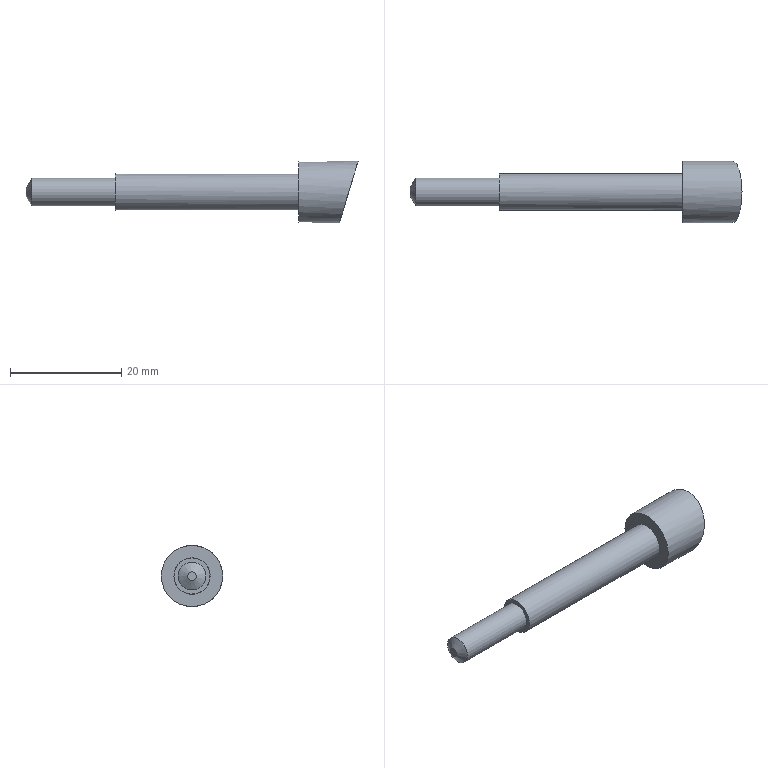Part | STEP file | solid 151 | 1 solid | 8 faces | box 59.59 x 11 x 11 mm | volume 2247 mm3 | plane 4 | cylinder 3 | cone 1 | commonest cylinder face diameters 5 x1 6.5 x1 11 x1